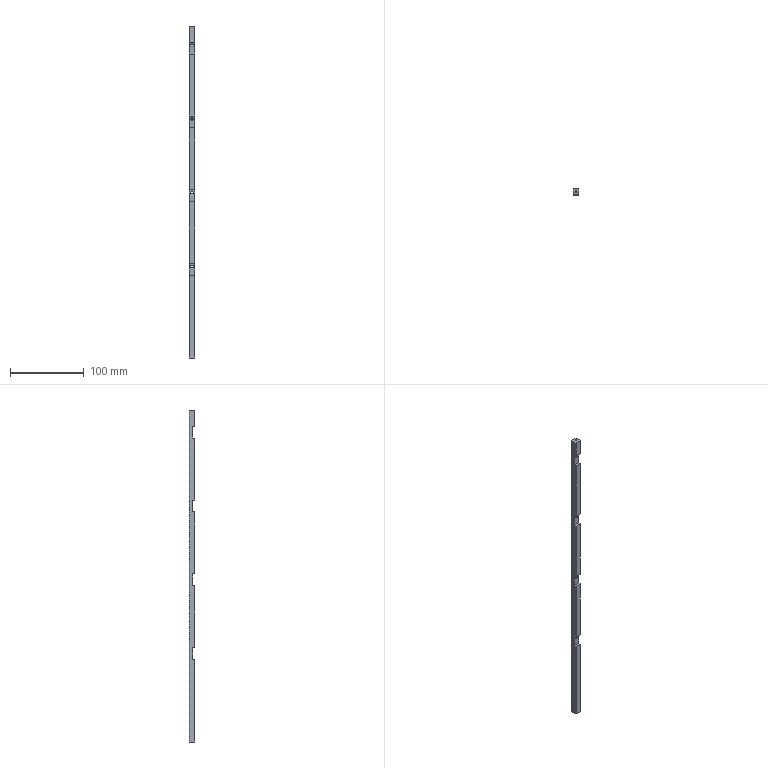Part | SolidWorks | features HoleWzd 3, ICE 2, Extrusion 1 | 1 solid | 50 faces | box 8 x 8 x 450 mm | volume 26809 mm3 | plane 26 | cylinder 20 | cone 4 | commonest cylinder face diameters 3.4 x8 6 x8 2.5 x4
STEP:
#1=CARTESIAN_POINT('',(0.,2.,121.));
#2=VERTEX_POINT('',#1);
#3=CARTESIAN_POINT('',(0.,2.,127.));
#4=VERTEX_POINT('',#3);
#5=CARTESIAN_POINT('',(0.,2.,124.));
#6=DIRECTION('',(0.,1.,0.));
#7=DIRECTION('',(0.,0.,1.));
#8=AXIS2_PLACEMENT_3D('',#5,#6,#7);
#9=CIRCLE('',#8,3.);
#10=EDGE_CURVE('',#2,#4,#9,.T.);
#11=ORIENTED_EDGE('',*,*,#10,.F.);
#12=CARTESIAN_POINT('',(0.,4.,121.));
#13=VERTEX_POINT('',#12);
#14=CARTESIAN_POINT('',(0.,4.,121.));
#15=DIRECTION('',(0.,1.,0.));
#16=VECTOR('',#15,1000.);
#17=LINE('',#14,#16);
#18=EDGE_CURVE('',#2,#13,#17,.T.);
#19=ORIENTED_EDGE('',*,*,#18,.T.);
#20=CARTESIAN_POINT('',(0.,4.,127.));
#21=VERTEX_POINT('',#20);
#22=CARTESIAN_POINT('',(0.,4.,124.));
#23=DIRECTION('',(0.,1.,0.));
#24=DIRECTION('',(0.,0.,1.));
#25=AXIS2_PLACEMENT_3D('',#22,#23,#24);
#26=CIRCLE('',#25,3.);
#27=EDGE_CURVE('',#13,#21,#26,.T.);
#28=ORIENTED_EDGE('',*,*,#27,.T.);
#29=CARTESIAN_POINT('',(0.,4.,127.));
#30=DIRECTION('',(0.,1.,0.));
#31=VECTOR('',#30,1000.);
#32=LINE('',#29,#31);
#33=EDGE_CURVE('',#4,#21,#32,.T.);
#34=ORIENTED_EDGE('',*,*,#33,.F.);
#35=EDGE_LOOP('',(#11,#19,#28,#34));
#36=FACE_OUTER_BOUND('',#35,.T.);
#37=CARTESIAN_POINT('',(0.,4.,124.));
#38=DIRECTION('',(0.,1.,0.));
#39=DIRECTION('',(0.,0.,1.));
#40=AXIS2_PLACEMENT_3D('',#37,#38,#39);
#41=CYLINDRICAL_SURFACE('',#40,3.);
#42=ADVANCED_FACE('',(#36),#41,.F.);
#43=CARTESIAN_POINT('',(0.,-1.,122.3));
#44=VERTEX_POINT('',#43);
#45=CARTESIAN_POINT('',(0.,-1.,125.7));
#46=VERTEX_POINT('',#45);
#47=CARTESIAN_POINT('',(0.,-1.,124.));
#48=DIRECTION('',(0.,1.,0.));
#49=DIRECTION('',(-1.,0.,0.));
#50=AXIS2_PLACEMENT_3D('',#47,#48,#49);
#51=CIRCLE('',#50,1.7);
#52=EDGE_CURVE('',#44,#46,#51,.T.);
#53=ORIENTED_EDGE('',*,*,#52,.F.);
#54=CARTESIAN_POINT('',(0.,2.,122.3));
#55=VERTEX_POINT('',#54);
#56=CARTESIAN_POINT('',(0.,4.,122.3));
#57=DIRECTION('',(0.,1.,0.));
#58=VECTOR('',#57,1000.);
#59=LINE('',#56,#58);
#60=EDGE_CURVE('',#44,#55,#59,.T.);
#61=ORIENTED_EDGE('',*,*,#60,.T.);
#62=CARTESIAN_POINT('',(0.,2.,125.7));
#63=VERTEX_POINT('',#62);
#64=CARTESIAN_POINT('',(0.,2.,124.));
#65=DIRECTION('',(0.,1.,0.));
#66=DIRECTION('',(0.,0.,1.));
#67=AXIS2_PLACEMENT_3D('',#64,#65,#66);
#68=CIRCLE('',#67,1.7);
#69=EDGE_CURVE('',#55,#63,#68,.T.);
#70=ORIENTED_EDGE('',*,*,#69,.T.);
#71=CARTESIAN_POINT('',(0.,4.,125.7));
#72=DIRECTION('',(0.,1.,0.));
#73=VECTOR('',#72,1000.);
#74=LINE('',#71,#73);
#75=EDGE_CURVE('',#46,#63,#74,.T.);
#76=ORIENTED_EDGE('',*,*,#75,.F.);
#77=EDGE_LOOP('',(#53,#61,#70,#76));
#78=FACE_OUTER_BOUND('',#77,.T.);
#79=CARTESIAN_POINT('',(0.,4.,124.));
#80=DIRECTION('',(0.,1.,0.));
#81=DIRECTION('',(0.,0.,1.));
#82=AXIS2_PLACEMENT_3D('',#79,#80,#81);
#83=CYLINDRICAL_SURFACE('',#82,1.7);
#84=ADVANCED_FACE('',(#78),#83,.F.);
#85=CARTESIAN_POINT('',(0.,2.,221.));
#86=VERTEX_POINT('',#85);
#87=CARTESIAN_POINT('',(0.,2.,227.));
#88=VERTEX_POINT('',#87);
#89=CARTESIAN_POINT('',(0.,2.,224.));
#90=DIRECTION('',(0.,1.,0.));
#91=DIRECTION('',(0.,0.,1.));
#92=AXIS2_PLACEMENT_3D('',#89,#90,#91);
#93=CIRCLE('',#92,3.);
#94=EDGE_CURVE('',#86,#88,#93,.T.);
#95=ORIENTED_EDGE('',*,*,#94,.F.);
#96=CARTESIAN_POINT('',(0.,4.,221.));
#97=VERTEX_POINT('',#96);
#98=CARTESIAN_POINT('',(0.,4.,221.));
#99=DIRECTION('',(0.,1.,0.));
#100=VECTOR('',#99,1000.);
#101=LINE('',#98,#100);
#102=EDGE_CURVE('',#86,#97,#101,.T.);
#103=ORIENTED_EDGE('',*,*,#102,.T.);
#104=CARTESIAN_POINT('',(0.,4.,227.));
#105=VERTEX_POINT('',#104);
#106=CARTESIAN_POINT('',(0.,4.,224.));
#107=DIRECTION('',(0.,1.,0.));
#108=DIRECTION('',(0.,0.,1.));
#109=AXIS2_PLACEMENT_3D('',#106,#107,#108);
#110=CIRCLE('',#109,3.);
#111=EDGE_CURVE('',#97,#105,#110,.T.);
#112=ORIENTED_EDGE('',*,*,#111,.T.);
#113=CARTESIAN_POINT('',(0.,4.,227.));
#114=DIRECTION('',(0.,1.,0.));
#115=VECTOR('',#114,1000.);
#116=LINE('',#113,#115);
#117=EDGE_CURVE('',#88,#105,#116,.T.);
#118=ORIENTED_EDGE('',*,*,#117,.F.);
#119=EDGE_LOOP('',(#95,#103,#112,#118));
#120=FACE_OUTER_BOUND('',#119,.T.);
#121=CARTESIAN_POINT('',(0.,4.,224.));
#122=DIRECTION('',(0.,1.,0.));
#123=DIRECTION('',(0.,0.,1.));
#124=AXIS2_PLACEMENT_3D('',#121,#122,#123);
#125=CYLINDRICAL_SURFACE('',#124,3.);
#126=ADVANCED_FACE('',(#120),#125,.F.);
#127=CARTESIAN_POINT('',(0.,-1.,222.3));
#128=VERTEX_POINT('',#127);
#129=CARTESIAN_POINT('',(0.,-1.,225.7));
#130=VERTEX_POINT('',#129);
#131=CARTESIAN_POINT('',(0.,-1.,224.));
#132=DIRECTION('',(0.,1.,0.));
#133=DIRECTION('',(-1.,0.,0.));
#134=AXIS2_PLACEMENT_3D('',#131,#132,#133);
#135=CIRCLE('',#134,1.7);
#136=EDGE_CURVE('',#128,#130,#135,.T.);
#137=ORIENTED_EDGE('',*,*,#136,.F.);
#138=CARTESIAN_POINT('',(0.,2.,222.3));
#139=VERTEX_POINT('',#138);
#140=CARTESIAN_POINT('',(0.,4.,222.3));
#141=DIRECTION('',(0.,1.,0.));
#142=VECTOR('',#141,1000.);
#143=LINE('',#140,#142);
#144=EDGE_CURVE('',#128,#139,#143,.T.);
#145=ORIENTED_EDGE('',*,*,#144,.T.);
#146=CARTESIAN_POINT('',(0.,2.,225.7));
#147=VERTEX_POINT('',#146);
#148=CARTESIAN_POINT('',(0.,2.,224.));
#149=DIRECTION('',(0.,1.,0.));
#150=DIRECTION('',(0.,0.,1.));
#151=AXIS2_PLACEMENT_3D('',#148,#149,#150);
#152=CIRCLE('',#151,1.7);
#153=EDGE_CURVE('',#139,#147,#152,.T.);
#154=ORIENTED_EDGE('',*,*,#153,.T.);
#155=CARTESIAN_POINT('',(0.,4.,225.7));
#156=DIRECTION('',(0.,1.,0.));
#157=VECTOR('',#156,1000.);
#158=LINE('',#155,#157);
#159=EDGE_CURVE('',#130,#147,#158,.T.);
#160=ORIENTED_EDGE('',*,*,#159,.F.);
#161=EDGE_LOOP('',(#137,#145,#154,#160));
#162=FACE_OUTER_BOUND('',#161,.T.);
#163=CARTESIAN_POINT('',(0.,4.,224.));
#164=DIRECTION('',(0.,1.,0.));
#165=DIRECTION('',(0.,0.,1.));
#166=AXIS2_PLACEMENT_3D('',#163,#164,#165);
#167=CYLINDRICAL_SURFACE('',#166,1.7);
#168=ADVANCED_FACE('',(#162),#167,.F.);
#169=CARTESIAN_POINT('',(0.,2.,321.));
#170=VERTEX_POINT('',#169);
#171=CARTESIAN_POINT('',(0.,2.,327.));
#172=VERTEX_POINT('',#171);
#173=CARTESIAN_POINT('',(0.,2.,324.));
#174=DIRECTION('',(0.,1.,0.));
#175=DIRECTION('',(0.,0.,1.));
#176=AXIS2_PLACEMENT_3D('',#173,#174,#175);
#177=CIRCLE('',#176,3.);
#178=EDGE_CURVE('',#170,#172,#177,.T.);
#179=ORIENTED_EDGE('',*,*,#178,.F.);
#180=CARTESIAN_POINT('',(0.,4.,321.));
#181=VERTEX_POINT('',#180);
#182=CARTESIAN_POINT('',(0.,4.,321.));
#183=DIRECTION('',(0.,1.,0.));
#184=VECTOR('',#183,1000.);
#185=LINE('',#182,#184);
#186=EDGE_CURVE('',#170,#181,#185,.T.);
#187=ORIENTED_EDGE('',*,*,#186,.T.);
#188=CARTESIAN_POINT('',(0.,4.,327.));
#189=VERTEX_POINT('',#188);
#190=CARTESIAN_POINT('',(0.,4.,324.));
#191=DIRECTION('',(0.,1.,0.));
#192=DIRECTION('',(0.,0.,1.));
#193=AXIS2_PLACEMENT_3D('',#190,#191,#192);
#194=CIRCLE('',#193,3.);
#195=EDGE_CURVE('',#181,#189,#194,.T.);
#196=ORIENTED_EDGE('',*,*,#195,.T.);
#197=CARTESIAN_POINT('',(0.,4.,327.));
#198=DIRECTION('',(0.,1.,0.));
#199=VECTOR('',#198,1000.);
#200=LINE('',#197,#199);
#201=EDGE_CURVE('',#172,#189,#200,.T.);
#202=ORIENTED_EDGE('',*,*,#201,.F.);
#203=EDGE_LOOP('',(#179,#187,#196,#202));
#204=FACE_OUTER_BOUND('',#203,.T.);
#205=CARTESIAN_POINT('',(0.,4.,324.));
#206=DIRECTION('',(0.,1.,0.));
#207=DIRECTION('',(0.,0.,1.));
#208=AXIS2_PLACEMENT_3D('',#205,#206,#207);
#209=CYLINDRICAL_SURFACE('',#208,3.);
#210=ADVANCED_FACE('',(#204),#209,.F.);
#211=CARTESIAN_POINT('',(0.,-1.,322.3));
#212=VERTEX_POINT('',#211);
#213=CARTESIAN_POINT('',(0.,-1.,325.7));
#214=VERTEX_POINT('',#213);
#215=CARTESIAN_POINT('',(0.,-1.,324.));
#216=DIRECTION('',(0.,1.,0.));
#217=DIRECTION('',(0.,0.,1.));
#218=AXIS2_PLACEMENT_3D('',#215,#216,#217);
#219=CIRCLE('',#218,1.7);
#220=EDGE_CURVE('',#212,#214,#219,.T.);
#221=ORIENTED_EDGE('',*,*,#220,.F.);
#222=CARTESIAN_POINT('',(0.,2.,322.3));
#223=VERTEX_POINT('',#222);
#224=CARTESIAN_POINT('',(0.,4.,322.3));
#225=DIRECTION('',(0.,1.,0.));
#226=VECTOR('',#225,1000.);
#227=LINE('',#224,#226);
#228=EDGE_CURVE('',#212,#223,#227,.T.);
#229=ORIENTED_EDGE('',*,*,#228,.T.);
#230=CARTESIAN_POINT('',(0.,2.,325.7));
#231=VERTEX_POINT('',#230);
#232=CARTESIAN_POINT('',(0.,2.,324.));
#233=DIRECTION('',(0.,1.,0.));
#234=DIRECTION('',(0.,0.,1.));
#235=AXIS2_PLACEMENT_3D('',#232,#233,#234);
#236=CIRCLE('',#235,1.7);
#237=EDGE_CURVE('',#223,#231,#236,.T.);
#238=ORIENTED_EDGE('',*,*,#237,.T.);
#239=CARTESIAN_POINT('',(0.,4.,325.7));
#240=DIRECTION('',(0.,1.,0.));
#241=VECTOR('',#240,1000.);
#242=LINE('',#239,#241);
#243=EDGE_CURVE('',#214,#231,#242,.T.);
#244=ORIENTED_EDGE('',*,*,#243,.F.);
#245=EDGE_LOOP('',(#221,#229,#238,#244));
#246=FACE_OUTER_BOUND('',#245,.T.);
#247=CARTESIAN_POINT('',(0.,4.,324.));
#248=DIRECTION('',(0.,1.,0.));
#249=DIRECTION('',(0.,0.,1.));
#250=AXIS2_PLACEMENT_3D('',#247,#248,#249);
#251=CYLINDRICAL_SURFACE('',#250,1.7);
#252=ADVANCED_FACE('',(#246),#251,.F.);
#253=CARTESIAN_POINT('',(0.,2.,421.));
#254=VERTEX_POINT('',#253);
#255=CARTESIAN_POINT('',(0.,2.,427.));
#256=VERTEX_POINT('',#255);
#257=CARTESIAN_POINT('',(0.,2.,424.));
#258=DIRECTION('',(0.,1.,0.));
#259=DIRECTION('',(0.,0.,1.));
#260=AXIS2_PLACEMENT_3D('',#257,#258,#259);
#261=CIRCLE('',#260,3.);
#262=EDGE_CURVE('',#254,#256,#261,.T.);
#263=ORIENTED_EDGE('',*,*,#262,.F.);
#264=CARTESIAN_POINT('',(0.,4.,421.));
#265=VERTEX_POINT('',#264);
#266=CARTESIAN_POINT('',(0.,4.,421.));
#267=DIRECTION('',(0.,1.,0.));
#268=VECTOR('',#267,1000.);
#269=LINE('',#266,#268);
#270=EDGE_CURVE('',#254,#265,#269,.T.);
#271=ORIENTED_EDGE('',*,*,#270,.T.);
#272=CARTESIAN_POINT('',(0.,4.,427.));
#273=VERTEX_POINT('',#272);
#274=CARTESIAN_POINT('',(0.,4.,424.));
#275=DIRECTION('',(0.,1.,0.));
#276=DIRECTION('',(0.,0.,1.));
#277=AXIS2_PLACEMENT_3D('',#274,#275,#276);
#278=CIRCLE('',#277,3.);
#279=EDGE_CURVE('',#265,#273,#278,.T.);
#280=ORIENTED_EDGE('',*,*,#279,.T.);
#281=CARTESIAN_POINT('',(0.,4.,427.));
#282=DIRECTION('',(0.,1.,0.));
#283=VECTOR('',#282,1000.);
#284=LINE('',#281,#283);
#285=EDGE_CURVE('',#256,#273,#284,.T.);
#286=ORIENTED_EDGE('',*,*,#285,.F.);
#287=EDGE_LOOP('',(#263,#271,#280,#286));
#288=FACE_OUTER_BOUND('',#287,.T.);
#289=CARTESIAN_POINT('',(0.,4.,424.));
#290=DIRECTION('',(0.,1.,0.));
#291=DIRECTION('',(0.,0.,1.));
#292=AXIS2_PLACEMENT_3D('',#289,#290,#291);
#293=CYLINDRICAL_SURFACE('',#292,3.);
#294=ADVANCED_FACE('',(#288),#293,.F.);
#295=CARTESIAN_POINT('',(0.,-1.,425.7));
#296=VERTEX_POINT('',#295);
#297=CARTESIAN_POINT('',(0.,-1.,422.3));
#298=VERTEX_POINT('',#297);
#299=CARTESIAN_POINT('',(0.,-1.,424.));
#300=DIRECTION('',(0.,-1.,0.));
#301=DIRECTION('',(0.,0.,-1.));
#302=AXIS2_PLACEMENT_3D('',#299,#300,#301);
#303=CIRCLE('',#302,1.7);
#304=EDGE_CURVE('',#296,#298,#303,.T.);
#305=ORIENTED_EDGE('',*,*,#304,.T.);
#306=CARTESIAN_POINT('',(0.,2.,422.3));
#307=VERTEX_POINT('',#306);
#308=CARTESIAN_POINT('',(0.,4.,422.3));
#309=DIRECTION('',(0.,1.,0.));
#310=VECTOR('',#309,1000.);
#311=LINE('',#308,#310);
#312=EDGE_CURVE('',#298,#307,#311,.T.);
#313=ORIENTED_EDGE('',*,*,#312,.T.);
#314=CARTESIAN_POINT('',(0.,2.,425.7));
#315=VERTEX_POINT('',#314);
#316=CARTESIAN_POINT('',(0.,2.,424.));
#317=DIRECTION('',(0.,1.,0.));
#318=DIRECTION('',(0.,0.,1.));
#319=AXIS2_PLACEMENT_3D('',#316,#317,#318);
#320=CIRCLE('',#319,1.7);
#321=EDGE_CURVE('',#307,#315,#320,.T.);
#322=ORIENTED_EDGE('',*,*,#321,.T.);
#323=CARTESIAN_POINT('',(0.,4.,425.7));
#324=DIRECTION('',(0.,1.,0.));
#325=VECTOR('',#324,1000.);
#326=LINE('',#323,#325);
#327=EDGE_CURVE('',#296,#315,#326,.T.);
#328=ORIENTED_EDGE('',*,*,#327,.F.);
#329=EDGE_LOOP('',(#305,#313,#322,#328));
#330=FACE_OUTER_BOUND('',#329,.T.);
#331=CARTESIAN_POINT('',(0.,4.,424.));
#332=DIRECTION('',(0.,1.,0.));
#333=DIRECTION('',(0.,0.,1.));
#334=AXIS2_PLACEMENT_3D('',#331,#332,#333);
#335=CYLINDRICAL_SURFACE('',#334,1.7);
#336=ADVANCED_FACE('',(#330),#335,.F.);
#337=CARTESIAN_POINT('',(-1.25,0.,438.));
#338=VERTEX_POINT('',#337);
#339=CARTESIAN_POINT('',(1.25,0.,438.));
#340=VERTEX_POINT('',#339);
#341=CARTESIAN_POINT('',(0.,0.,438.));
#342=DIRECTION('',(0.,0.,1.));
#343=DIRECTION('',(1.,0.,0.));
#344=AXIS2_PLACEMENT_3D('',#341,#342,#343);
#345=CIRCLE('',#344,1.25);
#346=EDGE_CURVE('',#338,#340,#345,.T.);
#347=ORIENTED_EDGE('',*,*,#346,.F.);
#348=CARTESIAN_POINT('',(-1.25,0.,450.));
#349=VERTEX_POINT('',#348);
#350=CARTESIAN_POINT('',(-1.25,0.,450.));
#351=DIRECTION('',(0.,0.,1.));
#352=VECTOR('',#351,1000.);
#353=LINE('',#350,#352);
#354=EDGE_CURVE('',#338,#349,#353,.T.);
#355=ORIENTED_EDGE('',*,*,#354,.T.);
#356=CARTESIAN_POINT('',(1.25,0.,450.));
#357=VERTEX_POINT('',#356);
#358=CARTESIAN_POINT('',(0.,0.,450.));
#359=DIRECTION('',(0.,0.,1.));
#360=DIRECTION('',(1.,0.,0.));
#361=AXIS2_PLACEMENT_3D('',#358,#359,#360);
#362=CIRCLE('',#361,1.25);
#363=EDGE_CURVE('',#349,#357,#362,.T.);
#364=ORIENTED_EDGE('',*,*,#363,.T.);
#365=CARTESIAN_POINT('',(1.25,0.,450.));
#366=DIRECTION('',(0.,0.,1.));
#367=VECTOR('',#366,1000.);
#368=LINE('',#365,#367);
#369=EDGE_CURVE('',#340,#357,#368,.T.);
#370=ORIENTED_EDGE('',*,*,#369,.F.);
#371=EDGE_LOOP('',(#347,#355,#364,#370));
#372=FACE_OUTER_BOUND('',#371,.T.);
#373=CARTESIAN_POINT('',(0.,0.,450.));
#374=DIRECTION('',(0.,0.,1.));
#375=DIRECTION('',(1.,0.,0.));
#376=AXIS2_PLACEMENT_3D('',#373,#374,#375);
#377=CYLINDRICAL_SURFACE('',#376,1.25);
#378=ADVANCED_FACE('',(#372),#377,.F.);
#379=CARTESIAN_POINT('',(0.,0.,437.249));
#380=VERTEX_POINT('',#379);
#381=CARTESIAN_POINT('',(1.25,0.,438.));
#382=DIRECTION('',(0.8572,0.,0.515));
#383=VECTOR('',#382,1000.);
#384=LINE('',#381,#383);
#385=EDGE_CURVE('',#380,#340,#384,.T.);
#386=ORIENTED_EDGE('',*,*,#385,.F.);
#387=CARTESIAN_POINT('',(-1.25,0.,438.));
#388=DIRECTION('',(-0.8572,0.,0.515));
#389=VECTOR('',#388,1000.);
#390=LINE('',#387,#389);
#391=EDGE_CURVE('',#380,#338,#390,.T.);
#392=ORIENTED_EDGE('',*,*,#391,.T.);
#393=ORIENTED_EDGE('',*,*,#346,.T.);
#394=EDGE_LOOP('',(#386,#392,#393));
#395=FACE_OUTER_BOUND('',#394,.T.);
#396=CARTESIAN_POINT('',(0.,0.,438.));
#397=DIRECTION('',(0.,0.,1.));
#398=DIRECTION('',(1.,0.,0.));
#399=AXIS2_PLACEMENT_3D('',#396,#397,#398);
#400=CONICAL_SURFACE('',#399,1.25,1.03);
#401=ADVANCED_FACE('',(#395),#400,.F.);
#402=CARTESIAN_POINT('',(1.25,0.,12.));
#403=VERTEX_POINT('',#402);
#404=CARTESIAN_POINT('',(-1.25,0.,12.));
#405=VERTEX_POINT('',#404);
#406=CARTESIAN_POINT('',(0.,0.,12.));
#407=DIRECTION('',(0.,0.,-1.));
#408=DIRECTION('',(-1.,0.,0.));
#409=AXIS2_PLACEMENT_3D('',#406,#407,#408);
#410=CIRCLE('',#409,1.25);
#411=EDGE_CURVE('',#403,#405,#410,.T.);
#412=ORIENTED_EDGE('',*,*,#411,.F.);
#413=CARTESIAN_POINT('',(1.25,0.,0.));
#414=VERTEX_POINT('',#413);
#415=CARTESIAN_POINT('',(1.25,0.,0.));
#416=DIRECTION('',(0.,0.,-1.));
#417=VECTOR('',#416,1000.);
#418=LINE('',#415,#417);
#419=EDGE_CURVE('',#403,#414,#418,.T.);
#420=ORIENTED_EDGE('',*,*,#419,.T.);
#421=CARTESIAN_POINT('',(-1.25,0.,0.));
#422=VERTEX_POINT('',#421);
#423=CARTESIAN_POINT('',(0.,0.,0.));
#424=DIRECTION('',(0.,0.,-1.));
#425=DIRECTION('',(-1.,0.,0.));
#426=AXIS2_PLACEMENT_3D('',#423,#424,#425);
#427=CIRCLE('',#426,1.25);
#428=EDGE_CURVE('',#414,#422,#427,.T.);
#429=ORIENTED_EDGE('',*,*,#428,.T.);
#430=CARTESIAN_POINT('',(-1.25,0.,0.));
#431=DIRECTION('',(0.,0.,-1.));
#432=VECTOR('',#431,1000.);
#433=LINE('',#430,#432);
#434=EDGE_CURVE('',#405,#422,#433,.T.);
#435=ORIENTED_EDGE('',*,*,#434,.F.);
#436=EDGE_LOOP('',(#412,#420,#429,#435));
#437=FACE_OUTER_BOUND('',#436,.T.);
#438=CARTESIAN_POINT('',(0.,0.,0.));
#439=DIRECTION('',(0.,0.,-1.));
#440=DIRECTION('',(-1.,0.,0.));
#441=AXIS2_PLACEMENT_3D('',#438,#439,#440);
#442=CYLINDRICAL_SURFACE('',#441,1.25);
#443=ADVANCED_FACE('',(#437),#442,.F.);
#444=CARTESIAN_POINT('',(0.,0.,12.751));
#445=VERTEX_POINT('',#444);
#446=CARTESIAN_POINT('',(-1.25,0.,12.));
#447=DIRECTION('',(-0.8572,0.,-0.515));
#448=VECTOR('',#447,1000.);
#449=LINE('',#446,#448);
#450=EDGE_CURVE('',#445,#405,#449,.T.);
#451=ORIENTED_EDGE('',*,*,#450,.F.);
#452=CARTESIAN_POINT('',(1.25,0.,12.));
#453=DIRECTION('',(0.8572,0.,-0.515));
#454=VECTOR('',#453,1000.);
#455=LINE('',#452,#454);
#456=EDGE_CURVE('',#445,#403,#455,.T.);
#457=ORIENTED_EDGE('',*,*,#456,.T.);
#458=ORIENTED_EDGE('',*,*,#411,.T.);
#459=EDGE_LOOP('',(#451,#457,#458));
#460=FACE_OUTER_BOUND('',#459,.T.);
#461=CARTESIAN_POINT('',(0.,0.,12.));
#462=DIRECTION('',(0.,0.,-1.));
#463=DIRECTION('',(-1.,0.,0.));
#464=AXIS2_PLACEMENT_3D('',#461,#462,#463);
#465=CONICAL_SURFACE('',#464,1.25,1.03);
#466=ADVANCED_FACE('',(#460),#465,.F.);
#467=CARTESIAN_POINT('',(-4.,-4.,212.));
#468=VERTEX_POINT('',#467);
#469=CARTESIAN_POINT('',(-4.,-4.,128.));
#470=VERTEX_POINT('',#469);
#471=CARTESIAN_POINT('',(-4.,-4.,450.));
#472=DIRECTION('',(0.,0.,-1.));
#473=VECTOR('',#472,1000.);
#474=LINE('',#471,#473);
#475=EDGE_CURVE('',#468,#470,#474,.T.);
#476=ORIENTED_EDGE('',*,*,#475,.T.);
#477=CARTESIAN_POINT('',(4.,-4.,128.));
#478=VERTEX_POINT('',#477);
#479=CARTESIAN_POINT('',(-4.,-4.,128.));
#480=DIRECTION('',(1.,0.,0.));
#481=VECTOR('',#480,1000.);
#482=LINE('',#479,#481);
#483=EDGE_CURVE('',#470,#478,#482,.T.);
#484=ORIENTED_EDGE('',*,*,#483,.T.);
#485=CARTESIAN_POINT('',(4.,-4.,212.));
#486=VERTEX_POINT('',#485);
#487=CARTESIAN_POINT('',(4.,-4.,450.));
#488=DIRECTION('',(0.,0.,-1.));
#489=VECTOR('',#488,1000.);
#490=LINE('',#487,#489);
#491=EDGE_CURVE('',#486,#478,#490,.T.);
#492=ORIENTED_EDGE('',*,*,#491,.F.);
#493=CARTESIAN_POINT('',(-4.,-4.,212.));
#494=DIRECTION('',(1.,0.,0.));
#495=VECTOR('',#494,1000.);
#496=LINE('',#493,#495);
#497=EDGE_CURVE('',#468,#486,#496,.T.);
#498=ORIENTED_EDGE('',*,*,#497,.F.);
#499=EDGE_LOOP('',(#476,#484,#492,#498));
#500=FACE_OUTER_BOUND('',#499,.T.);
#501=CARTESIAN_POINT('',(-4.,-4.,450.));
#502=DIRECTION('',(0.,1.,0.));
#503=DIRECTION('',(0.,0.,1.));
#504=AXIS2_PLACEMENT_3D('',#501,#502,#503);
#505=PLANE('',#504);
#506=ADVANCED_FACE('',(#500),#505,.F.);
#507=CARTESIAN_POINT('',(-4.,-4.,312.));
#508=VERTEX_POINT('',#507);
#509=CARTESIAN_POINT('',(-4.,-4.,228.));
#510=VERTEX_POINT('',#509);
#511=CARTESIAN_POINT('',(-4.,-4.,450.));
#512=DIRECTION('',(0.,0.,-1.));
#513=VECTOR('',#512,1000.);
#514=LINE('',#511,#513);
#515=EDGE_CURVE('',#508,#510,#514,.T.);
#516=ORIENTED_EDGE('',*,*,#515,.T.);
#517=CARTESIAN_POINT('',(4.,-4.,228.));
#518=VERTEX_POINT('',#517);
#519=CARTESIAN_POINT('',(-4.,-4.,228.));
#520=DIRECTION('',(1.,0.,0.));
#521=VECTOR('',#520,1000.);
#522=LINE('',#519,#521);
#523=EDGE_CURVE('',#510,#518,#522,.T.);
#524=ORIENTED_EDGE('',*,*,#523,.T.);
#525=CARTESIAN_POINT('',(4.,-4.,312.));
#526=VERTEX_POINT('',#525);
#527=CARTESIAN_POINT('',(4.,-4.,450.));
#528=DIRECTION('',(0.,0.,-1.));
#529=VECTOR('',#528,1000.);
#530=LINE('',#527,#529);
#531=EDGE_CURVE('',#526,#518,#530,.T.);
#532=ORIENTED_EDGE('',*,*,#531,.F.);
#533=CARTESIAN_POINT('',(-4.,-4.,312.));
#534=DIRECTION('',(1.,0.,0.));
#535=VECTOR('',#534,1000.);
#536=LINE('',#533,#535);
#537=EDGE_CURVE('',#508,#526,#536,.T.);
#538=ORIENTED_EDGE('',*,*,#537,.F.);
#539=EDGE_LOOP('',(#516,#524,#532,#538));
#540=FACE_OUTER_BOUND('',#539,.T.);
#541=CARTESIAN_POINT('',(-4.,-4.,450.));
#542=DIRECTION('',(0.,1.,0.));
#543=DIRECTION('',(0.,0.,1.));
#544=AXIS2_PLACEMENT_3D('',#541,#542,#543);
#545=PLANE('',#544);
#546=ADVANCED_FACE('',(#540),#545,.F.);
#547=CARTESIAN_POINT('',(4.,-4.,112.));
#548=VERTEX_POINT('',#547);
#549=CARTESIAN_POINT('',(4.,-4.,0.));
#550=VERTEX_POINT('',#549);
#551=CARTESIAN_POINT('',(4.,-4.,450.));
#552=DIRECTION('',(0.,0.,-1.));
#553=VECTOR('',#552,1000.);
#554=LINE('',#551,#553);
#555=EDGE_CURVE('',#548,#550,#554,.T.);
#556=ORIENTED_EDGE('',*,*,#555,.F.);
#557=CARTESIAN_POINT('',(-4.,-4.,112.));
#558=VERTEX_POINT('',#557);
#559=CARTESIAN_POINT('',(-4.,-4.,112.));
#560=DIRECTION('',(1.,0.,0.));
#561=VECTOR('',#560,1000.);
#562=LINE('',#559,#561);
#563=EDGE_CURVE('',#558,#548,#562,.T.);
#564=ORIENTED_EDGE('',*,*,#563,.F.);
#565=CARTESIAN_POINT('',(-4.,-4.,0.));
#566=VERTEX_POINT('',#565);
#567=CARTESIAN_POINT('',(-4.,-4.,450.));
#568=DIRECTION('',(0.,0.,-1.));
#569=VECTOR('',#568,1000.);
#570=LINE('',#567,#569);
#571=EDGE_CURVE('',#558,#566,#570,.T.);
#572=ORIENTED_EDGE('',*,*,#571,.T.);
#573=CARTESIAN_POINT('',(-4.,-4.,0.));
#574=DIRECTION('',(1.,0.,0.));
#575=VECTOR('',#574,1000.);
#576=LINE('',#573,#575);
#577=EDGE_CURVE('',#566,#550,#576,.T.);
#578=ORIENTED_EDGE('',*,*,#577,.T.);
#579=EDGE_LOOP('',(#556,#564,#572,#578));
#580=FACE_OUTER_BOUND('',#579,.T.);
#581=CARTESIAN_POINT('',(-4.,-4.,450.));
#582=DIRECTION('',(0.,1.,0.));
#583=DIRECTION('',(0.,0.,1.));
#584=AXIS2_PLACEMENT_3D('',#581,#582,#583);
#585=PLANE('',#584);
#586=ADVANCED_FACE('',(#580),#585,.F.);
#587=CARTESIAN_POINT('',(-4.,-4.,450.));
#588=VERTEX_POINT('',#587);
#589=CARTESIAN_POINT('',(-4.,-4.,428.));
#590=VERTEX_POINT('',#589);
#591=CARTESIAN_POINT('',(-4.,-4.,450.));
#592=DIRECTION('',(0.,0.,-1.));
#593=VECTOR('',#592,1000.);
#594=LINE('',#591,#593);
#595=EDGE_CURVE('',#588,#590,#594,.T.);
#596=ORIENTED_EDGE('',*,*,#595,.T.);
#597=CARTESIAN_POINT('',(4.,-4.,428.));
#598=VERTEX_POINT('',#597);
#599=CARTESIAN_POINT('',(-4.,-4.,428.));
#600=DIRECTION('',(-1.,0.,0.));
#601=VECTOR('',#600,1000.);
#602=LINE('',#599,#601);
#603=EDGE_CURVE('',#598,#590,#602,.T.);
#604=ORIENTED_EDGE('',*,*,#603,.F.);
#605=CARTESIAN_POINT('',(4.,-4.,450.));
#606=VERTEX_POINT('',#605);
#607=CARTESIAN_POINT('',(4.,-4.,450.));
#608=DIRECTION('',(0.,0.,-1.));
#609=VECTOR('',#608,1000.);
#610=LINE('',#607,#609);
#611=EDGE_CURVE('',#606,#598,#610,.T.);
#612=ORIENTED_EDGE('',*,*,#611,.F.);
#613=CARTESIAN_POINT('',(-4.,-4.,450.));
#614=DIRECTION('',(1.,0.,0.));
#615=VECTOR('',#614,1000.);
#616=LINE('',#613,#615);
#617=EDGE_CURVE('',#588,#606,#616,.T.);
#618=ORIENTED_EDGE('',*,*,#617,.F.);
#619=EDGE_LOOP('',(#596,#604,#612,#618));
#620=FACE_OUTER_BOUND('',#619,.T.);
#621=CARTESIAN_POINT('',(-4.,-4.,450.));
#622=DIRECTION('',(0.,1.,0.));
#623=DIRECTION('',(0.,0.,1.));
#624=AXIS2_PLACEMENT_3D('',#621,#622,#623);
#625=PLANE('',#624);
#626=ADVANCED_FACE('',(#620),#625,.F.);
#627=ORIENTED_EDGE('',*,*,#491,.T.);
#628=CARTESIAN_POINT('',(4.,-1.,128.));
#629=VERTEX_POINT('',#628);
#630=CARTESIAN_POINT('',(4.,-4.,128.));
#631=DIRECTION('',(0.,-1.,0.));
#632=VECTOR('',#631,1000.);
#633=LINE('',#630,#632);
#634=EDGE_CURVE('',#629,#478,#633,.T.);
#635=ORIENTED_EDGE('',*,*,#634,.F.);
#636=CARTESIAN_POINT('',(4.,-1.,112.));
#637=VERTEX_POINT('',#636);
#638=CARTESIAN_POINT('',(4.,-1.,128.));
#639=DIRECTION('',(0.,0.,1.));
#640=VECTOR('',#639,1000.);
#641=LINE('',#638,#640);
#642=EDGE_CURVE('',#637,#629,#641,.T.);
#643=ORIENTED_EDGE('',*,*,#642,.F.);
#644=CARTESIAN_POINT('',(4.,-4.,112.));
#645=DIRECTION('',(0.,1.,0.));
#646=VECTOR('',#645,1000.);
#647=LINE('',#644,#646);
#648=EDGE_CURVE('',#548,#637,#647,.T.);
#649=ORIENTED_EDGE('',*,*,#648,.F.);
#650=ORIENTED_EDGE('',*,*,#555,.T.);
#651=CARTESIAN_POINT('',(4.,4.,0.));
#652=VERTEX_POINT('',#651);
#653=CARTESIAN_POINT('',(4.,4.,0.));
#654=DIRECTION('',(0.,1.,0.));
#655=VECTOR('',#654,1000.);
#656=LINE('',#653,#655);
#657=EDGE_CURVE('',#550,#652,#656,.T.);
#658=ORIENTED_EDGE('',*,*,#657,.T.);
#659=CARTESIAN_POINT('',(4.,4.,450.));
#660=VERTEX_POINT('',#659);
#661=CARTESIAN_POINT('',(4.,4.,450.));
#662=DIRECTION('',(0.,0.,-1.));
#663=VECTOR('',#662,1000.);
#664=LINE('',#661,#663);
#665=EDGE_CURVE('',#660,#652,#664,.T.);
#666=ORIENTED_EDGE('',*,*,#665,.F.);
#667=CARTESIAN_POINT('',(4.,4.,450.));
#668=DIRECTION('',(0.,1.,0.));
#669=VECTOR('',#668,1000.);
#670=LINE('',#667,#669);
#671=EDGE_CURVE('',#606,#660,#670,.T.);
#672=ORIENTED_EDGE('',*,*,#671,.F.);
#673=ORIENTED_EDGE('',*,*,#611,.T.);
#674=CARTESIAN_POINT('',(4.,-1.,428.));
#675=VERTEX_POINT('',#674);
#676=CARTESIAN_POINT('',(4.,-1.,428.));
#677=DIRECTION('',(0.,-1.,0.));
#678=VECTOR('',#677,1000.);
#679=LINE('',#676,#678);
#680=EDGE_CURVE('',#675,#598,#679,.T.);
#681=ORIENTED_EDGE('',*,*,#680,.F.);
#682=CARTESIAN_POINT('',(4.,-1.,412.));
#683=VERTEX_POINT('',#682);
#684=CARTESIAN_POINT('',(4.,-1.,428.));
#685=DIRECTION('',(0.,0.,1.));
#686=VECTOR('',#685,1000.);
#687=LINE('',#684,#686);
#688=EDGE_CURVE('',#683,#675,#687,.T.);
#689=ORIENTED_EDGE('',*,*,#688,.F.);
#690=CARTESIAN_POINT('',(4.,-4.,412.));
#691=VERTEX_POINT('',#690);
#692=CARTESIAN_POINT('',(4.,-1.,412.));
#693=DIRECTION('',(0.,-1.,0.));
#694=VECTOR('',#693,1000.);
#695=LINE('',#692,#694);
#696=EDGE_CURVE('',#683,#691,#695,.T.);
#697=ORIENTED_EDGE('',*,*,#696,.T.);
#698=CARTESIAN_POINT('',(4.,-4.,328.));
#699=VERTEX_POINT('',#698);
#700=CARTESIAN_POINT('',(4.,-4.,450.));
#701=DIRECTION('',(0.,0.,-1.));
#702=VECTOR('',#701,1000.);
#703=LINE('',#700,#702);
#704=EDGE_CURVE('',#691,#699,#703,.T.);
#705=ORIENTED_EDGE('',*,*,#704,.T.);
#706=CARTESIAN_POINT('',(4.,-1.,328.));
#707=VERTEX_POINT('',#706);
#708=CARTESIAN_POINT('',(4.,-4.,328.));
#709=DIRECTION('',(0.,-1.,0.));
#710=VECTOR('',#709,1000.);
#711=LINE('',#708,#710);
#712=EDGE_CURVE('',#707,#699,#711,.T.);
#713=ORIENTED_EDGE('',*,*,#712,.F.);
#714=CARTESIAN_POINT('',(4.,-1.,312.));
#715=VERTEX_POINT('',#714);
#716=CARTESIAN_POINT('',(4.,-1.,312.));
#717=DIRECTION('',(0.,0.,1.));
#718=VECTOR('',#717,1000.);
#719=LINE('',#716,#718);
#720=EDGE_CURVE('',#715,#707,#719,.T.);
#721=ORIENTED_EDGE('',*,*,#720,.F.);
#722=CARTESIAN_POINT('',(4.,-4.,312.));
#723=DIRECTION('',(0.,1.,0.));
#724=VECTOR('',#723,1000.);
#725=LINE('',#722,#724);
#726=EDGE_CURVE('',#526,#715,#725,.T.);
#727=ORIENTED_EDGE('',*,*,#726,.F.);
#728=ORIENTED_EDGE('',*,*,#531,.T.);
#729=CARTESIAN_POINT('',(4.,-1.,228.));
#730=VERTEX_POINT('',#729);
#731=CARTESIAN_POINT('',(4.,-4.,228.));
#732=DIRECTION('',(0.,-1.,0.));
#733=VECTOR('',#732,1000.);
#734=LINE('',#731,#733);
#735=EDGE_CURVE('',#730,#518,#734,.T.);
#736=ORIENTED_EDGE('',*,*,#735,.F.);
#737=CARTESIAN_POINT('',(4.,-1.,212.));
#738=VERTEX_POINT('',#737);
#739=CARTESIAN_POINT('',(4.,-1.,228.));
#740=DIRECTION('',(0.,0.,1.));
#741=VECTOR('',#740,1000.);
#742=LINE('',#739,#741);
#743=EDGE_CURVE('',#738,#730,#742,.T.);
#744=ORIENTED_EDGE('',*,*,#743,.F.);
#745=CARTESIAN_POINT('',(4.,-4.,212.));
#746=DIRECTION('',(0.,1.,0.));
#747=VECTOR('',#746,1000.);
#748=LINE('',#745,#747);
#749=EDGE_CURVE('',#486,#738,#748,.T.);
#750=ORIENTED_EDGE('',*,*,#749,.F.);
#751=EDGE_LOOP('',(#627,#635,#643,#649,#650,#658,#666,#672,#673,#681,#689,#697,#705,#713,#721,#727,#728,#736,#744,#750));
#752=FACE_OUTER_BOUND('',#751,.T.);
#753=CARTESIAN_POINT('',(4.,4.,450.));
#754=DIRECTION('',(-1.,0.,0.));
#755=DIRECTION('',(0.,-1.,0.));
#756=AXIS2_PLACEMENT_3D('',#753,#754,#755);
#757=PLANE('',#756);
#758=ADVANCED_FACE('',(#752),#757,.F.);
#759=CARTESIAN_POINT('',(0.,4.,124.));
#760=DIRECTION('',(0.,1.,0.));
#761=DIRECTION('',(0.,0.,1.));
#762=AXIS2_PLACEMENT_3D('',#759,#760,#761);
#763=CIRCLE('',#762,3.);
#764=EDGE_CURVE('',#21,#13,#763,.T.);
#765=ORIENTED_EDGE('',*,*,#764,.F.);
#766=ORIENTED_EDGE('',*,*,#27,.F.);
#767=EDGE_LOOP('',(#765,#766));
#768=FACE_BOUND('',#767,.T.);
#769=CARTESIAN_POINT('',(0.,4.,224.));
#770=DIRECTION('',(0.,1.,0.));
#771=DIRECTION('',(0.,0.,1.));
#772=AXIS2_PLACEMENT_3D('',#769,#770,#771);
#773=CIRCLE('',#772,3.);
#774=EDGE_CURVE('',#105,#97,#773,.T.);
#775=ORIENTED_EDGE('',*,*,#774,.F.);
#776=ORIENTED_EDGE('',*,*,#111,.F.);
#777=EDGE_LOOP('',(#775,#776));
#778=FACE_BOUND('',#777,.T.);
#779=CARTESIAN_POINT('',(0.,4.,324.));
#780=DIRECTION('',(0.,1.,0.));
#781=DIRECTION('',(0.,0.,1.));
#782=AXIS2_PLACEMENT_3D('',#779,#780,#781);
#783=CIRCLE('',#782,3.);
#784=EDGE_CURVE('',#189,#181,#783,.T.);
#785=ORIENTED_EDGE('',*,*,#784,.F.);
#786=ORIENTED_EDGE('',*,*,#195,.F.);
#787=EDGE_LOOP('',(#785,#786));
#788=FACE_BOUND('',#787,.T.);
#789=CARTESIAN_POINT('',(0.,4.,424.));
#790=DIRECTION('',(0.,1.,0.));
#791=DIRECTION('',(0.,0.,1.));
#792=AXIS2_PLACEMENT_3D('',#789,#790,#791);
#793=CIRCLE('',#792,3.);
#794=EDGE_CURVE('',#273,#265,#793,.T.);
#795=ORIENTED_EDGE('',*,*,#794,.F.);
#796=ORIENTED_EDGE('',*,*,#279,.F.);
#797=EDGE_LOOP('',(#795,#796));
#798=FACE_BOUND('',#797,.T.);
#799=CARTESIAN_POINT('',(-4.,4.,0.));
#800=VERTEX_POINT('',#799);
#801=CARTESIAN_POINT('',(-4.,4.,0.));
#802=DIRECTION('',(-1.,0.,0.));
#803=VECTOR('',#802,1000.);
#804=LINE('',#801,#803);
#805=EDGE_CURVE('',#652,#800,#804,.T.);
#806=ORIENTED_EDGE('',*,*,#805,.T.);
#807=CARTESIAN_POINT('',(-4.,4.,450.));
#808=VERTEX_POINT('',#807);
#809=CARTESIAN_POINT('',(-4.,4.,450.));
#810=DIRECTION('',(0.,0.,-1.));
#811=VECTOR('',#810,1000.);
#812=LINE('',#809,#811);
#813=EDGE_CURVE('',#808,#800,#812,.T.);
#814=ORIENTED_EDGE('',*,*,#813,.F.);
#815=CARTESIAN_POINT('',(-4.,4.,450.));
#816=DIRECTION('',(-1.,0.,0.));
#817=VECTOR('',#816,1000.);
#818=LINE('',#815,#817);
#819=EDGE_CURVE('',#660,#808,#818,.T.);
#820=ORIENTED_EDGE('',*,*,#819,.F.);
#821=ORIENTED_EDGE('',*,*,#665,.T.);
#822=EDGE_LOOP('',(#806,#814,#820,#821));
#823=FACE_OUTER_BOUND('',#822,.T.);
#824=CARTESIAN_POINT('',(-4.,4.,450.));
#825=DIRECTION('',(0.,-1.,0.));
#826=DIRECTION('',(0.,0.,-1.));
#827=AXIS2_PLACEMENT_3D('',#824,#825,#826);
#828=PLANE('',#827);
#829=ADVANCED_FACE('',(#768,#778,#788,#798,#823),#828,.F.);
#830=CARTESIAN_POINT('',(-4.,-1.,112.));
#831=VERTEX_POINT('',#830);
#832=CARTESIAN_POINT('',(-4.,-1.,128.));
#833=VERTEX_POINT('',#832);
#834=CARTESIAN_POINT('',(-4.,-1.,128.));
#835=DIRECTION('',(0.,0.,1.));
#836=VECTOR('',#835,1000.);
#837=LINE('',#834,#836);
#838=EDGE_CURVE('',#831,#833,#837,.T.);
#839=ORIENTED_EDGE('',*,*,#838,.T.);
#840=CARTESIAN_POINT('',(-4.,-4.,128.));
#841=DIRECTION('',(0.,-1.,0.));
#842=VECTOR('',#841,1000.);
#843=LINE('',#840,#842);
#844=EDGE_CURVE('',#833,#470,#843,.T.);
#845=ORIENTED_EDGE('',*,*,#844,.T.);
#846=ORIENTED_EDGE('',*,*,#475,.F.);
#847=CARTESIAN_POINT('',(-4.,-1.,212.));
#848=VERTEX_POINT('',#847);
#849=CARTESIAN_POINT('',(-4.,-4.,212.));
#850=DIRECTION('',(0.,1.,0.));
#851=VECTOR('',#850,1000.);
#852=LINE('',#849,#851);
#853=EDGE_CURVE('',#468,#848,#852,.T.);
#854=ORIENTED_EDGE('',*,*,#853,.T.);
#855=CARTESIAN_POINT('',(-4.,-1.,228.));
#856=VERTEX_POINT('',#855);
#857=CARTESIAN_POINT('',(-4.,-1.,228.));
#858=DIRECTION('',(0.,0.,1.));
#859=VECTOR('',#858,1000.);
#860=LINE('',#857,#859);
#861=EDGE_CURVE('',#848,#856,#860,.T.);
#862=ORIENTED_EDGE('',*,*,#861,.T.);
#863=CARTESIAN_POINT('',(-4.,-4.,228.));
#864=DIRECTION('',(0.,-1.,0.));
#865=VECTOR('',#864,1000.);
#866=LINE('',#863,#865);
#867=EDGE_CURVE('',#856,#510,#866,.T.);
#868=ORIENTED_EDGE('',*,*,#867,.T.);
#869=ORIENTED_EDGE('',*,*,#515,.F.);
#870=CARTESIAN_POINT('',(-4.,-1.,312.));
#871=VERTEX_POINT('',#870);
#872=CARTESIAN_POINT('',(-4.,-4.,312.));
#873=DIRECTION('',(0.,1.,0.));
#874=VECTOR('',#873,1000.);
#875=LINE('',#872,#874);
#876=EDGE_CURVE('',#508,#871,#875,.T.);
#877=ORIENTED_EDGE('',*,*,#876,.T.);
#878=CARTESIAN_POINT('',(-4.,-1.,328.));
#879=VERTEX_POINT('',#878);
#880=CARTESIAN_POINT('',(-4.,-1.,312.));
#881=DIRECTION('',(0.,0.,1.));
#882=VECTOR('',#881,1000.);
#883=LINE('',#880,#882);
#884=EDGE_CURVE('',#871,#879,#883,.T.);
#885=ORIENTED_EDGE('',*,*,#884,.T.);
#886=CARTESIAN_POINT('',(-4.,-4.,328.));
#887=VERTEX_POINT('',#886);
#888=CARTESIAN_POINT('',(-4.,-4.,328.));
#889=DIRECTION('',(0.,-1.,0.));
#890=VECTOR('',#889,1000.);
#891=LINE('',#888,#890);
#892=EDGE_CURVE('',#879,#887,#891,.T.);
#893=ORIENTED_EDGE('',*,*,#892,.T.);
#894=CARTESIAN_POINT('',(-4.,-4.,412.));
#895=VERTEX_POINT('',#894);
#896=CARTESIAN_POINT('',(-4.,-4.,450.));
#897=DIRECTION('',(0.,0.,-1.));
#898=VECTOR('',#897,1000.);
#899=LINE('',#896,#898);
#900=EDGE_CURVE('',#895,#887,#899,.T.);
#901=ORIENTED_EDGE('',*,*,#900,.F.);
#902=CARTESIAN_POINT('',(-4.,-1.,412.));
#903=VERTEX_POINT('',#902);
#904=CARTESIAN_POINT('',(-4.,-1.,412.));
#905=DIRECTION('',(0.,-1.,0.));
#906=VECTOR('',#905,1000.);
#907=LINE('',#904,#906);
#908=EDGE_CURVE('',#903,#895,#907,.T.);
#909=ORIENTED_EDGE('',*,*,#908,.F.);
#910=CARTESIAN_POINT('',(-4.,-1.,428.));
#911=VERTEX_POINT('',#910);
#912=CARTESIAN_POINT('',(-4.,-1.,428.));
#913=DIRECTION('',(0.,0.,-1.));
#914=VECTOR('',#913,1000.);
#915=LINE('',#912,#914);
#916=EDGE_CURVE('',#911,#903,#915,.T.);
#917=ORIENTED_EDGE('',*,*,#916,.F.);
#918=CARTESIAN_POINT('',(-4.,-1.,428.));
#919=DIRECTION('',(0.,-1.,0.));
#920=VECTOR('',#919,1000.);
#921=LINE('',#918,#920);
#922=EDGE_CURVE('',#911,#590,#921,.T.);
#923=ORIENTED_EDGE('',*,*,#922,.T.);
#924=ORIENTED_EDGE('',*,*,#595,.F.);
#925=CARTESIAN_POINT('',(-4.,4.,450.));
#926=DIRECTION('',(0.,-1.,0.));
#927=VECTOR('',#926,1000.);
#928=LINE('',#925,#927);
#929=EDGE_CURVE('',#808,#588,#928,.T.);
#930=ORIENTED_EDGE('',*,*,#929,.F.);
#931=ORIENTED_EDGE('',*,*,#813,.T.);
#932=CARTESIAN_POINT('',(-4.,4.,0.));
#933=DIRECTION('',(0.,-1.,0.));
#934=VECTOR('',#933,1000.);
#935=LINE('',#932,#934);
#936=EDGE_CURVE('',#800,#566,#935,.T.);
#937=ORIENTED_EDGE('',*,*,#936,.T.);
#938=ORIENTED_EDGE('',*,*,#571,.F.);
#939=CARTESIAN_POINT('',(-4.,-4.,112.));
#940=DIRECTION('',(0.,1.,0.));
#941=VECTOR('',#940,1000.);
#942=LINE('',#939,#941);
#943=EDGE_CURVE('',#558,#831,#942,.T.);
#944=ORIENTED_EDGE('',*,*,#943,.T.);
#945=EDGE_LOOP('',(#839,#845,#846,#854,#862,#868,#869,#877,#885,#893,#901,#909,#917,#923,#924,#930,#931,#937,#938,#944));
#946=FACE_OUTER_BOUND('',#945,.T.);
#947=CARTESIAN_POINT('',(-4.,4.,450.));
#948=DIRECTION('',(1.,0.,0.));
#949=DIRECTION('',(0.,1.,0.));
#950=AXIS2_PLACEMENT_3D('',#947,#948,#949);
#951=PLANE('',#950);
#952=ADVANCED_FACE('',(#946),#951,.F.);
#953=ORIENTED_EDGE('',*,*,#900,.T.);
#954=CARTESIAN_POINT('',(-4.,-4.,328.));
#955=DIRECTION('',(1.,0.,0.));
#956=VECTOR('',#955,1000.);
#957=LINE('',#954,#956);
#958=EDGE_CURVE('',#887,#699,#957,.T.);
#959=ORIENTED_EDGE('',*,*,#958,.T.);
#960=ORIENTED_EDGE('',*,*,#704,.F.);
#961=CARTESIAN_POINT('',(-4.,-4.,412.));
#962=DIRECTION('',(1.,0.,0.));
#963=VECTOR('',#962,1000.);
#964=LINE('',#961,#963);
#965=EDGE_CURVE('',#895,#691,#964,.T.);
#966=ORIENTED_EDGE('',*,*,#965,.F.);
#967=EDGE_LOOP('',(#953,#959,#960,#966));
#968=FACE_OUTER_BOUND('',#967,.T.);
#969=CARTESIAN_POINT('',(-4.,-4.,450.));
#970=DIRECTION('',(0.,1.,0.));
#971=DIRECTION('',(0.,0.,1.));
#972=AXIS2_PLACEMENT_3D('',#969,#970,#971);
#973=PLANE('',#972);
#974=ADVANCED_FACE('',(#968),#973,.F.);
#975=CARTESIAN_POINT('',(0.,0.,450.));
#976=DIRECTION('',(0.,0.,1.));
#977=DIRECTION('',(1.,0.,0.));
#978=AXIS2_PLACEMENT_3D('',#975,#976,#977);
#979=CIRCLE('',#978,1.25);
#980=EDGE_CURVE('',#357,#349,#979,.T.);
#981=ORIENTED_EDGE('',*,*,#980,.F.);
#982=ORIENTED_EDGE('',*,*,#363,.F.);
#983=EDGE_LOOP('',(#981,#982));
#984=FACE_BOUND('',#983,.T.);
#985=ORIENTED_EDGE('',*,*,#671,.T.);
#986=ORIENTED_EDGE('',*,*,#819,.T.);
#987=ORIENTED_EDGE('',*,*,#929,.T.);
#988=ORIENTED_EDGE('',*,*,#617,.T.);
#989=EDGE_LOOP('',(#985,#986,#987,#988));
#990=FACE_OUTER_BOUND('',#989,.T.);
#991=CARTESIAN_POINT('',(0.,0.,450.));
#992=DIRECTION('',(0.,0.,1.));
#993=DIRECTION('',(1.,0.,0.));
#994=AXIS2_PLACEMENT_3D('',#991,#992,#993);
#995=PLANE('',#994);
#996=ADVANCED_FACE('',(#984,#990),#995,.T.);
#997=CARTESIAN_POINT('',(0.,0.,0.));
#998=DIRECTION('',(0.,0.,-1.));
#999=DIRECTION('',(-1.,0.,0.));
#1000=AXIS2_PLACEMENT_3D('',#997,#998,#999);
#1001=CIRCLE('',#1000,1.25);
#1002=EDGE_CURVE('',#422,#414,#1001,.T.);
#1003=ORIENTED_EDGE('',*,*,#1002,.F.);
#1004=ORIENTED_EDGE('',*,*,#428,.F.);
#1005=EDGE_LOOP('',(#1003,#1004));
#1006=FACE_BOUND('',#1005,.T.);
#1007=ORIENTED_EDGE('',*,*,#657,.F.);
#1008=ORIENTED_EDGE('',*,*,#577,.F.);
#1009=ORIENTED_EDGE('',*,*,#936,.F.);
#1010=ORIENTED_EDGE('',*,*,#805,.F.);
#1011=EDGE_LOOP('',(#1007,#1008,#1009,#1010));
#1012=FACE_OUTER_BOUND('',#1011,.T.);
#1013=CARTESIAN_POINT('',(0.,0.,0.));
#1014=DIRECTION('',(0.,0.,1.));
#1015=DIRECTION('',(1.,0.,0.));
#1016=AXIS2_PLACEMENT_3D('',#1013,#1014,#1015);
#1017=PLANE('',#1016);
#1018=ADVANCED_FACE('',(#1006,#1012),#1017,.F.);
#1019=ORIENTED_EDGE('',*,*,#603,.T.);
#1020=ORIENTED_EDGE('',*,*,#922,.F.);
#1021=CARTESIAN_POINT('',(-4.,-1.,428.));
#1022=DIRECTION('',(-1.,0.,0.));
#1023=VECTOR('',#1022,1000.);
#1024=LINE('',#1021,#1023);
#1025=EDGE_CURVE('',#675,#911,#1024,.T.);
#1026=ORIENTED_EDGE('',*,*,#1025,.F.);
#1027=ORIENTED_EDGE('',*,*,#680,.T.);
#1028=EDGE_LOOP('',(#1019,#1020,#1026,#1027));
#1029=FACE_OUTER_BOUND('',#1028,.T.);
#1030=CARTESIAN_POINT('',(-4.,-1.,428.));
#1031=DIRECTION('',(0.,0.,1.));
#1032=DIRECTION('',(1.,0.,0.));
#1033=AXIS2_PLACEMENT_3D('',#1030,#1031,#1032);
#1034=PLANE('',#1033);
#1035=ADVANCED_FACE('',(#1029),#1034,.F.);
#1036=ORIENTED_EDGE('',*,*,#965,.T.);
#1037=ORIENTED_EDGE('',*,*,#696,.F.);
#1038=CARTESIAN_POINT('',(-4.,-1.,412.));
#1039=DIRECTION('',(1.,0.,0.));
#1040=VECTOR('',#1039,1000.);
#1041=LINE('',#1038,#1040);
#1042=EDGE_CURVE('',#903,#683,#1041,.T.);
#1043=ORIENTED_EDGE('',*,*,#1042,.F.);
#1044=ORIENTED_EDGE('',*,*,#908,.T.);
#1045=EDGE_LOOP('',(#1036,#1037,#1043,#1044));
#1046=FACE_OUTER_BOUND('',#1045,.T.);
#1047=CARTESIAN_POINT('',(-4.,-1.,412.));
#1048=DIRECTION('',(0.,0.,-1.));
#1049=DIRECTION('',(-1.,0.,0.));
#1050=AXIS2_PLACEMENT_3D('',#1047,#1048,#1049);
#1051=PLANE('',#1050);
#1052=ADVANCED_FACE('',(#1046),#1051,.F.);
#1053=ORIENTED_EDGE('',*,*,#304,.F.);
#1054=CARTESIAN_POINT('',(0.,-1.,424.));
#1055=DIRECTION('',(0.,-1.,0.));
#1056=DIRECTION('',(0.,0.,-1.));
#1057=AXIS2_PLACEMENT_3D('',#1054,#1055,#1056);
#1058=CIRCLE('',#1057,1.7);
#1059=EDGE_CURVE('',#298,#296,#1058,.T.);
#1060=ORIENTED_EDGE('',*,*,#1059,.F.);
#1061=EDGE_LOOP('',(#1053,#1060));
#1062=FACE_BOUND('',#1061,.T.);
#1063=ORIENTED_EDGE('',*,*,#916,.T.);
#1064=ORIENTED_EDGE('',*,*,#1042,.T.);
#1065=ORIENTED_EDGE('',*,*,#688,.T.);
#1066=ORIENTED_EDGE('',*,*,#1025,.T.);
#1067=EDGE_LOOP('',(#1063,#1064,#1065,#1066));
#1068=FACE_OUTER_BOUND('',#1067,.T.);
#1069=CARTESIAN_POINT('',(0.,-1.,0.));
#1070=DIRECTION('',(0.,-1.,0.));
#1071=DIRECTION('',(0.,0.,-1.));
#1072=AXIS2_PLACEMENT_3D('',#1069,#1070,#1071);
#1073=PLANE('',#1072);
#1074=ADVANCED_FACE('',(#1062,#1068),#1073,.T.);
#1075=ORIENTED_EDGE('',*,*,#456,.F.);
#1076=ORIENTED_EDGE('',*,*,#450,.T.);
#1077=CARTESIAN_POINT('',(0.,0.,12.));
#1078=DIRECTION('',(0.,0.,-1.));
#1079=DIRECTION('',(-1.,0.,0.));
#1080=AXIS2_PLACEMENT_3D('',#1077,#1078,#1079);
#1081=CIRCLE('',#1080,1.25);
#1082=EDGE_CURVE('',#405,#403,#1081,.T.);
#1083=ORIENTED_EDGE('',*,*,#1082,.T.);
#1084=EDGE_LOOP('',(#1075,#1076,#1083));
#1085=FACE_OUTER_BOUND('',#1084,.T.);
#1086=CARTESIAN_POINT('',(0.,0.,12.));
#1087=DIRECTION('',(0.,0.,-1.));
#1088=DIRECTION('',(-1.,0.,0.));
#1089=AXIS2_PLACEMENT_3D('',#1086,#1087,#1088);
#1090=CONICAL_SURFACE('',#1089,1.25,1.03);
#1091=ADVANCED_FACE('',(#1085),#1090,.F.);
#1092=ORIENTED_EDGE('',*,*,#419,.F.);
#1093=ORIENTED_EDGE('',*,*,#1082,.F.);
#1094=ORIENTED_EDGE('',*,*,#434,.T.);
#1095=ORIENTED_EDGE('',*,*,#1002,.T.);
#1096=EDGE_LOOP('',(#1092,#1093,#1094,#1095));
#1097=FACE_OUTER_BOUND('',#1096,.T.);
#1098=CARTESIAN_POINT('',(0.,0.,0.));
#1099=DIRECTION('',(0.,0.,-1.));
#1100=DIRECTION('',(-1.,0.,0.));
#1101=AXIS2_PLACEMENT_3D('',#1098,#1099,#1100);
#1102=CYLINDRICAL_SURFACE('',#1101,1.25);
#1103=ADVANCED_FACE('',(#1097),#1102,.F.);
#1104=ORIENTED_EDGE('',*,*,#391,.F.);
#1105=ORIENTED_EDGE('',*,*,#385,.T.);
#1106=CARTESIAN_POINT('',(0.,0.,438.));
#1107=DIRECTION('',(0.,0.,1.));
#1108=DIRECTION('',(1.,0.,0.));
#1109=AXIS2_PLACEMENT_3D('',#1106,#1107,#1108);
#1110=CIRCLE('',#1109,1.25);
#1111=EDGE_CURVE('',#340,#338,#1110,.T.);
#1112=ORIENTED_EDGE('',*,*,#1111,.T.);
#1113=EDGE_LOOP('',(#1104,#1105,#1112));
#1114=FACE_OUTER_BOUND('',#1113,.T.);
#1115=CARTESIAN_POINT('',(0.,0.,438.));
#1116=DIRECTION('',(0.,0.,1.));
#1117=DIRECTION('',(1.,0.,0.));
#1118=AXIS2_PLACEMENT_3D('',#1115,#1116,#1117);
#1119=CONICAL_SURFACE('',#1118,1.25,1.03);
#1120=ADVANCED_FACE('',(#1114),#1119,.F.);
#1121=ORIENTED_EDGE('',*,*,#354,.F.);
#1122=ORIENTED_EDGE('',*,*,#1111,.F.);
#1123=ORIENTED_EDGE('',*,*,#369,.T.);
#1124=ORIENTED_EDGE('',*,*,#980,.T.);
#1125=EDGE_LOOP('',(#1121,#1122,#1123,#1124));
#1126=FACE_OUTER_BOUND('',#1125,.T.);
#1127=CARTESIAN_POINT('',(0.,0.,450.));
#1128=DIRECTION('',(0.,0.,1.));
#1129=DIRECTION('',(1.,0.,0.));
#1130=AXIS2_PLACEMENT_3D('',#1127,#1128,#1129);
#1131=CYLINDRICAL_SURFACE('',#1130,1.25);
#1132=ADVANCED_FACE('',(#1126),#1131,.F.);
#1133=ORIENTED_EDGE('',*,*,#726,.T.);
#1134=CARTESIAN_POINT('',(-4.,-1.,312.));
#1135=DIRECTION('',(1.,0.,0.));
#1136=VECTOR('',#1135,1000.);
#1137=LINE('',#1134,#1136);
#1138=EDGE_CURVE('',#871,#715,#1137,.T.);
#1139=ORIENTED_EDGE('',*,*,#1138,.F.);
#1140=ORIENTED_EDGE('',*,*,#876,.F.);
#1141=ORIENTED_EDGE('',*,*,#537,.T.);
#1142=EDGE_LOOP('',(#1133,#1139,#1140,#1141));
#1143=FACE_OUTER_BOUND('',#1142,.T.);
#1144=CARTESIAN_POINT('',(-4.,-4.,312.));
#1145=DIRECTION('',(0.,0.,-1.));
#1146=DIRECTION('',(-1.,0.,0.));
#1147=AXIS2_PLACEMENT_3D('',#1144,#1145,#1146);
#1148=PLANE('',#1147);
#1149=ADVANCED_FACE('',(#1143),#1148,.F.);
#1150=ORIENTED_EDGE('',*,*,#712,.T.);
#1151=ORIENTED_EDGE('',*,*,#958,.F.);
#1152=ORIENTED_EDGE('',*,*,#892,.F.);
#1153=CARTESIAN_POINT('',(-4.,-1.,328.));
#1154=DIRECTION('',(1.,0.,0.));
#1155=VECTOR('',#1154,1000.);
#1156=LINE('',#1153,#1155);
#1157=EDGE_CURVE('',#879,#707,#1156,.T.);
#1158=ORIENTED_EDGE('',*,*,#1157,.T.);
#1159=EDGE_LOOP('',(#1150,#1151,#1152,#1158));
#1160=FACE_OUTER_BOUND('',#1159,.T.);
#1161=CARTESIAN_POINT('',(-4.,-4.,328.));
#1162=DIRECTION('',(0.,0.,1.));
#1163=DIRECTION('',(1.,0.,0.));
#1164=AXIS2_PLACEMENT_3D('',#1161,#1162,#1163);
#1165=PLANE('',#1164);
#1166=ADVANCED_FACE('',(#1160),#1165,.F.);
#1167=CARTESIAN_POINT('',(0.,-1.,324.));
#1168=DIRECTION('',(0.,1.,0.));
#1169=DIRECTION('',(0.,0.,1.));
#1170=AXIS2_PLACEMENT_3D('',#1167,#1168,#1169);
#1171=CIRCLE('',#1170,1.7);
#1172=EDGE_CURVE('',#214,#212,#1171,.T.);
#1173=ORIENTED_EDGE('',*,*,#1172,.T.);
#1174=ORIENTED_EDGE('',*,*,#220,.T.);
#1175=EDGE_LOOP('',(#1173,#1174));
#1176=FACE_BOUND('',#1175,.T.);
#1177=ORIENTED_EDGE('',*,*,#720,.T.);
#1178=ORIENTED_EDGE('',*,*,#1157,.F.);
#1179=ORIENTED_EDGE('',*,*,#884,.F.);
#1180=ORIENTED_EDGE('',*,*,#1138,.T.);
#1181=EDGE_LOOP('',(#1177,#1178,#1179,#1180));
#1182=FACE_OUTER_BOUND('',#1181,.T.);
#1183=CARTESIAN_POINT('',(-4.,-1.,312.));
#1184=DIRECTION('',(0.,1.,0.));
#1185=DIRECTION('',(0.,0.,1.));
#1186=AXIS2_PLACEMENT_3D('',#1183,#1184,#1185);
#1187=PLANE('',#1186);
#1188=ADVANCED_FACE('',(#1176,#1182),#1187,.F.);
#1189=ORIENTED_EDGE('',*,*,#735,.T.);
#1190=ORIENTED_EDGE('',*,*,#523,.F.);
#1191=ORIENTED_EDGE('',*,*,#867,.F.);
#1192=CARTESIAN_POINT('',(-4.,-1.,228.));
#1193=DIRECTION('',(1.,0.,0.));
#1194=VECTOR('',#1193,1000.);
#1195=LINE('',#1192,#1194);
#1196=EDGE_CURVE('',#856,#730,#1195,.T.);
#1197=ORIENTED_EDGE('',*,*,#1196,.T.);
#1198=EDGE_LOOP('',(#1189,#1190,#1191,#1197));
#1199=FACE_OUTER_BOUND('',#1198,.T.);
#1200=CARTESIAN_POINT('',(-4.,-4.,228.));
#1201=DIRECTION('',(0.,0.,1.));
#1202=DIRECTION('',(1.,0.,0.));
#1203=AXIS2_PLACEMENT_3D('',#1200,#1201,#1202);
#1204=PLANE('',#1203);
#1205=ADVANCED_FACE('',(#1199),#1204,.F.);
#1206=CARTESIAN_POINT('',(0.,-1.,224.));
#1207=DIRECTION('',(0.,1.,0.));
#1208=DIRECTION('',(-1.,0.,0.));
#1209=AXIS2_PLACEMENT_3D('',#1206,#1207,#1208);
#1210=CIRCLE('',#1209,1.7);
#1211=EDGE_CURVE('',#130,#128,#1210,.T.);
#1212=ORIENTED_EDGE('',*,*,#1211,.T.);
#1213=ORIENTED_EDGE('',*,*,#136,.T.);
#1214=EDGE_LOOP('',(#1212,#1213));
#1215=FACE_BOUND('',#1214,.T.);
#1216=ORIENTED_EDGE('',*,*,#743,.T.);
#1217=ORIENTED_EDGE('',*,*,#1196,.F.);
#1218=ORIENTED_EDGE('',*,*,#861,.F.);
#1219=CARTESIAN_POINT('',(-4.,-1.,212.));
#1220=DIRECTION('',(1.,0.,0.));
#1221=VECTOR('',#1220,1000.);
#1222=LINE('',#1219,#1221);
#1223=EDGE_CURVE('',#848,#738,#1222,.T.);
#1224=ORIENTED_EDGE('',*,*,#1223,.T.);
#1225=EDGE_LOOP('',(#1216,#1217,#1218,#1224));
#1226=FACE_OUTER_BOUND('',#1225,.T.);
#1227=CARTESIAN_POINT('',(-4.,-1.,228.));
#1228=DIRECTION('',(0.,1.,0.));
#1229=DIRECTION('',(-1.,0.,0.));
#1230=AXIS2_PLACEMENT_3D('',#1227,#1228,#1229);
#1231=PLANE('',#1230);
#1232=ADVANCED_FACE('',(#1215,#1226),#1231,.F.);
#1233=ORIENTED_EDGE('',*,*,#749,.T.);
#1234=ORIENTED_EDGE('',*,*,#1223,.F.);
#1235=ORIENTED_EDGE('',*,*,#853,.F.);
#1236=ORIENTED_EDGE('',*,*,#497,.T.);
#1237=EDGE_LOOP('',(#1233,#1234,#1235,#1236));
#1238=FACE_OUTER_BOUND('',#1237,.T.);
#1239=CARTESIAN_POINT('',(-4.,-4.,212.));
#1240=DIRECTION('',(0.,0.,-1.));
#1241=DIRECTION('',(-1.,0.,0.));
#1242=AXIS2_PLACEMENT_3D('',#1239,#1240,#1241);
#1243=PLANE('',#1242);
#1244=ADVANCED_FACE('',(#1238),#1243,.F.);
#1245=ORIENTED_EDGE('',*,*,#634,.T.);
#1246=ORIENTED_EDGE('',*,*,#483,.F.);
#1247=ORIENTED_EDGE('',*,*,#844,.F.);
#1248=CARTESIAN_POINT('',(-4.,-1.,128.));
#1249=DIRECTION('',(1.,0.,0.));
#1250=VECTOR('',#1249,1000.);
#1251=LINE('',#1248,#1250);
#1252=EDGE_CURVE('',#833,#629,#1251,.T.);
#1253=ORIENTED_EDGE('',*,*,#1252,.T.);
#1254=EDGE_LOOP('',(#1245,#1246,#1247,#1253));
#1255=FACE_OUTER_BOUND('',#1254,.T.);
#1256=CARTESIAN_POINT('',(-4.,-4.,128.));
#1257=DIRECTION('',(0.,0.,1.));
#1258=DIRECTION('',(1.,0.,0.));
#1259=AXIS2_PLACEMENT_3D('',#1256,#1257,#1258);
#1260=PLANE('',#1259);
#1261=ADVANCED_FACE('',(#1255),#1260,.F.);
#1262=CARTESIAN_POINT('',(0.,-1.,124.));
#1263=DIRECTION('',(0.,1.,0.));
#1264=DIRECTION('',(-1.,0.,0.));
#1265=AXIS2_PLACEMENT_3D('',#1262,#1263,#1264);
#1266=CIRCLE('',#1265,1.7);
#1267=EDGE_CURVE('',#46,#44,#1266,.T.);
#1268=ORIENTED_EDGE('',*,*,#1267,.T.);
#1269=ORIENTED_EDGE('',*,*,#52,.T.);
#1270=EDGE_LOOP('',(#1268,#1269));
#1271=FACE_BOUND('',#1270,.T.);
#1272=ORIENTED_EDGE('',*,*,#642,.T.);
#1273=ORIENTED_EDGE('',*,*,#1252,.F.);
#1274=ORIENTED_EDGE('',*,*,#838,.F.);
#1275=CARTESIAN_POINT('',(-4.,-1.,112.));
#1276=DIRECTION('',(1.,0.,0.));
#1277=VECTOR('',#1276,1000.);
#1278=LINE('',#1275,#1277);
#1279=EDGE_CURVE('',#831,#637,#1278,.T.);
#1280=ORIENTED_EDGE('',*,*,#1279,.T.);
#1281=EDGE_LOOP('',(#1272,#1273,#1274,#1280));
#1282=FACE_OUTER_BOUND('',#1281,.T.);
#1283=CARTESIAN_POINT('',(-4.,-1.,128.));
#1284=DIRECTION('',(0.,1.,0.));
#1285=DIRECTION('',(-1.,0.,0.));
#1286=AXIS2_PLACEMENT_3D('',#1283,#1284,#1285);
#1287=PLANE('',#1286);
#1288=ADVANCED_FACE('',(#1271,#1282),#1287,.F.);
#1289=ORIENTED_EDGE('',*,*,#648,.T.);
#1290=ORIENTED_EDGE('',*,*,#1279,.F.);
#1291=ORIENTED_EDGE('',*,*,#943,.F.);
#1292=ORIENTED_EDGE('',*,*,#563,.T.);
#1293=EDGE_LOOP('',(#1289,#1290,#1291,#1292));
#1294=FACE_OUTER_BOUND('',#1293,.T.);
#1295=CARTESIAN_POINT('',(-4.,-4.,112.));
#1296=DIRECTION('',(0.,0.,-1.));
#1297=DIRECTION('',(-1.,0.,0.));
#1298=AXIS2_PLACEMENT_3D('',#1295,#1296,#1297);
#1299=PLANE('',#1298);
#1300=ADVANCED_FACE('',(#1294),#1299,.F.);
#1301=ORIENTED_EDGE('',*,*,#312,.F.);
#1302=ORIENTED_EDGE('',*,*,#1059,.T.);
#1303=ORIENTED_EDGE('',*,*,#327,.T.);
#1304=CARTESIAN_POINT('',(0.,2.,424.));
#1305=DIRECTION('',(0.,1.,0.));
#1306=DIRECTION('',(0.,0.,1.));
#1307=AXIS2_PLACEMENT_3D('',#1304,#1305,#1306);
#1308=CIRCLE('',#1307,1.7);
#1309=EDGE_CURVE('',#315,#307,#1308,.T.);
#1310=ORIENTED_EDGE('',*,*,#1309,.T.);
#1311=EDGE_LOOP('',(#1301,#1302,#1303,#1310));
#1312=FACE_OUTER_BOUND('',#1311,.T.);
#1313=CARTESIAN_POINT('',(0.,4.,424.));
#1314=DIRECTION('',(0.,1.,0.));
#1315=DIRECTION('',(0.,0.,1.));
#1316=AXIS2_PLACEMENT_3D('',#1313,#1314,#1315);
#1317=CYLINDRICAL_SURFACE('',#1316,1.7);
#1318=ADVANCED_FACE('',(#1312),#1317,.F.);
#1319=ORIENTED_EDGE('',*,*,#1309,.F.);
#1320=ORIENTED_EDGE('',*,*,#321,.F.);
#1321=EDGE_LOOP('',(#1319,#1320));
#1322=FACE_BOUND('',#1321,.T.);
#1323=CARTESIAN_POINT('',(0.,2.,424.));
#1324=DIRECTION('',(0.,1.,0.));
#1325=DIRECTION('',(0.,0.,1.));
#1326=AXIS2_PLACEMENT_3D('',#1323,#1324,#1325);
#1327=CIRCLE('',#1326,3.);
#1328=EDGE_CURVE('',#256,#254,#1327,.T.);
#1329=ORIENTED_EDGE('',*,*,#1328,.T.);
#1330=ORIENTED_EDGE('',*,*,#262,.T.);
#1331=EDGE_LOOP('',(#1329,#1330));
#1332=FACE_OUTER_BOUND('',#1331,.T.);
#1333=CARTESIAN_POINT('',(1.7,2.,424.));
#1334=DIRECTION('',(0.,-1.,0.));
#1335=DIRECTION('',(0.,0.,-1.));
#1336=AXIS2_PLACEMENT_3D('',#1333,#1334,#1335);
#1337=PLANE('',#1336);
#1338=ADVANCED_FACE('',(#1322,#1332),#1337,.F.);
#1339=ORIENTED_EDGE('',*,*,#270,.F.);
#1340=ORIENTED_EDGE('',*,*,#1328,.F.);
#1341=ORIENTED_EDGE('',*,*,#285,.T.);
#1342=ORIENTED_EDGE('',*,*,#794,.T.);
#1343=EDGE_LOOP('',(#1339,#1340,#1341,#1342));
#1344=FACE_OUTER_BOUND('',#1343,.T.);
#1345=CARTESIAN_POINT('',(0.,4.,424.));
#1346=DIRECTION('',(0.,1.,0.));
#1347=DIRECTION('',(0.,0.,1.));
#1348=AXIS2_PLACEMENT_3D('',#1345,#1346,#1347);
#1349=CYLINDRICAL_SURFACE('',#1348,3.);
#1350=ADVANCED_FACE('',(#1344),#1349,.F.);
#1351=ORIENTED_EDGE('',*,*,#228,.F.);
#1352=ORIENTED_EDGE('',*,*,#1172,.F.);
#1353=ORIENTED_EDGE('',*,*,#243,.T.);
#1354=CARTESIAN_POINT('',(0.,2.,324.));
#1355=DIRECTION('',(0.,1.,0.));
#1356=DIRECTION('',(0.,0.,1.));
#1357=AXIS2_PLACEMENT_3D('',#1354,#1355,#1356);
#1358=CIRCLE('',#1357,1.7);
#1359=EDGE_CURVE('',#231,#223,#1358,.T.);
#1360=ORIENTED_EDGE('',*,*,#1359,.T.);
#1361=EDGE_LOOP('',(#1351,#1352,#1353,#1360));
#1362=FACE_OUTER_BOUND('',#1361,.T.);
#1363=CARTESIAN_POINT('',(0.,4.,324.));
#1364=DIRECTION('',(0.,1.,0.));
#1365=DIRECTION('',(0.,0.,1.));
#1366=AXIS2_PLACEMENT_3D('',#1363,#1364,#1365);
#1367=CYLINDRICAL_SURFACE('',#1366,1.7);
#1368=ADVANCED_FACE('',(#1362),#1367,.F.);
#1369=ORIENTED_EDGE('',*,*,#1359,.F.);
#1370=ORIENTED_EDGE('',*,*,#237,.F.);
#1371=EDGE_LOOP('',(#1369,#1370));
#1372=FACE_BOUND('',#1371,.T.);
#1373=CARTESIAN_POINT('',(0.,2.,324.));
#1374=DIRECTION('',(0.,1.,0.));
#1375=DIRECTION('',(0.,0.,1.));
#1376=AXIS2_PLACEMENT_3D('',#1373,#1374,#1375);
#1377=CIRCLE('',#1376,3.);
#1378=EDGE_CURVE('',#172,#170,#1377,.T.);
#1379=ORIENTED_EDGE('',*,*,#1378,.T.);
#1380=ORIENTED_EDGE('',*,*,#178,.T.);
#1381=EDGE_LOOP('',(#1379,#1380));
#1382=FACE_OUTER_BOUND('',#1381,.T.);
#1383=CARTESIAN_POINT('',(1.7,2.,324.));
#1384=DIRECTION('',(0.,-1.,0.));
#1385=DIRECTION('',(0.,0.,-1.));
#1386=AXIS2_PLACEMENT_3D('',#1383,#1384,#1385);
#1387=PLANE('',#1386);
#1388=ADVANCED_FACE('',(#1372,#1382),#1387,.F.);
#1389=ORIENTED_EDGE('',*,*,#186,.F.);
#1390=ORIENTED_EDGE('',*,*,#1378,.F.);
#1391=ORIENTED_EDGE('',*,*,#201,.T.);
#1392=ORIENTED_EDGE('',*,*,#784,.T.);
#1393=EDGE_LOOP('',(#1389,#1390,#1391,#1392));
#1394=FACE_OUTER_BOUND('',#1393,.T.);
#1395=CARTESIAN_POINT('',(0.,4.,324.));
#1396=DIRECTION('',(0.,1.,0.));
#1397=DIRECTION('',(0.,0.,1.));
#1398=AXIS2_PLACEMENT_3D('',#1395,#1396,#1397);
#1399=CYLINDRICAL_SURFACE('',#1398,3.);
#1400=ADVANCED_FACE('',(#1394),#1399,.F.);
#1401=ORIENTED_EDGE('',*,*,#144,.F.);
#1402=ORIENTED_EDGE('',*,*,#1211,.F.);
#1403=ORIENTED_EDGE('',*,*,#159,.T.);
#1404=CARTESIAN_POINT('',(0.,2.,224.));
#1405=DIRECTION('',(0.,1.,0.));
#1406=DIRECTION('',(0.,0.,1.));
#1407=AXIS2_PLACEMENT_3D('',#1404,#1405,#1406);
#1408=CIRCLE('',#1407,1.7);
#1409=EDGE_CURVE('',#147,#139,#1408,.T.);
#1410=ORIENTED_EDGE('',*,*,#1409,.T.);
#1411=EDGE_LOOP('',(#1401,#1402,#1403,#1410));
#1412=FACE_OUTER_BOUND('',#1411,.T.);
#1413=CARTESIAN_POINT('',(0.,4.,224.));
#1414=DIRECTION('',(0.,1.,0.));
#1415=DIRECTION('',(0.,0.,1.));
#1416=AXIS2_PLACEMENT_3D('',#1413,#1414,#1415);
#1417=CYLINDRICAL_SURFACE('',#1416,1.7);
#1418=ADVANCED_FACE('',(#1412),#1417,.F.);
#1419=ORIENTED_EDGE('',*,*,#1409,.F.);
#1420=ORIENTED_EDGE('',*,*,#153,.F.);
#1421=EDGE_LOOP('',(#1419,#1420));
#1422=FACE_BOUND('',#1421,.T.);
#1423=CARTESIAN_POINT('',(0.,2.,224.));
#1424=DIRECTION('',(0.,1.,0.));
#1425=DIRECTION('',(0.,0.,1.));
#1426=AXIS2_PLACEMENT_3D('',#1423,#1424,#1425);
#1427=CIRCLE('',#1426,3.);
#1428=EDGE_CURVE('',#88,#86,#1427,.T.);
#1429=ORIENTED_EDGE('',*,*,#1428,.T.);
#1430=ORIENTED_EDGE('',*,*,#94,.T.);
#1431=EDGE_LOOP('',(#1429,#1430));
#1432=FACE_OUTER_BOUND('',#1431,.T.);
#1433=CARTESIAN_POINT('',(1.7,2.,224.));
#1434=DIRECTION('',(0.,-1.,0.));
#1435=DIRECTION('',(0.,0.,-1.));
#1436=AXIS2_PLACEMENT_3D('',#1433,#1434,#1435);
#1437=PLANE('',#1436);
#1438=ADVANCED_FACE('',(#1422,#1432),#1437,.F.);
#1439=ORIENTED_EDGE('',*,*,#102,.F.);
#1440=ORIENTED_EDGE('',*,*,#1428,.F.);
#1441=ORIENTED_EDGE('',*,*,#117,.T.);
#1442=ORIENTED_EDGE('',*,*,#774,.T.);
#1443=EDGE_LOOP('',(#1439,#1440,#1441,#1442));
#1444=FACE_OUTER_BOUND('',#1443,.T.);
#1445=CARTESIAN_POINT('',(0.,4.,224.));
#1446=DIRECTION('',(0.,1.,0.));
#1447=DIRECTION('',(0.,0.,1.));
#1448=AXIS2_PLACEMENT_3D('',#1445,#1446,#1447);
#1449=CYLINDRICAL_SURFACE('',#1448,3.);
#1450=ADVANCED_FACE('',(#1444),#1449,.F.);
#1451=ORIENTED_EDGE('',*,*,#60,.F.);
#1452=ORIENTED_EDGE('',*,*,#1267,.F.);
#1453=ORIENTED_EDGE('',*,*,#75,.T.);
#1454=CARTESIAN_POINT('',(0.,2.,124.));
#1455=DIRECTION('',(0.,1.,0.));
#1456=DIRECTION('',(0.,0.,1.));
#1457=AXIS2_PLACEMENT_3D('',#1454,#1455,#1456);
#1458=CIRCLE('',#1457,1.7);
#1459=EDGE_CURVE('',#63,#55,#1458,.T.);
#1460=ORIENTED_EDGE('',*,*,#1459,.T.);
#1461=EDGE_LOOP('',(#1451,#1452,#1453,#1460));
#1462=FACE_OUTER_BOUND('',#1461,.T.);
#1463=CARTESIAN_POINT('',(0.,4.,124.));
#1464=DIRECTION('',(0.,1.,0.));
#1465=DIRECTION('',(0.,0.,1.));
#1466=AXIS2_PLACEMENT_3D('',#1463,#1464,#1465);
#1467=CYLINDRICAL_SURFACE('',#1466,1.7);
#1468=ADVANCED_FACE('',(#1462),#1467,.F.);
#1469=ORIENTED_EDGE('',*,*,#1459,.F.);
#1470=ORIENTED_EDGE('',*,*,#69,.F.);
#1471=EDGE_LOOP('',(#1469,#1470));
#1472=FACE_BOUND('',#1471,.T.);
#1473=CARTESIAN_POINT('',(0.,2.,124.));
#1474=DIRECTION('',(0.,1.,0.));
#1475=DIRECTION('',(0.,0.,1.));
#1476=AXIS2_PLACEMENT_3D('',#1473,#1474,#1475);
#1477=CIRCLE('',#1476,3.);
#1478=EDGE_CURVE('',#4,#2,#1477,.T.);
#1479=ORIENTED_EDGE('',*,*,#1478,.T.);
#1480=ORIENTED_EDGE('',*,*,#10,.T.);
#1481=EDGE_LOOP('',(#1479,#1480));
#1482=FACE_OUTER_BOUND('',#1481,.T.);
#1483=CARTESIAN_POINT('',(1.7,2.,124.));
#1484=DIRECTION('',(0.,-1.,0.));
#1485=DIRECTION('',(0.,0.,-1.));
#1486=AXIS2_PLACEMENT_3D('',#1483,#1484,#1485);
#1487=PLANE('',#1486);
#1488=ADVANCED_FACE('',(#1472,#1482),#1487,.F.);
#1489=ORIENTED_EDGE('',*,*,#18,.F.);
#1490=ORIENTED_EDGE('',*,*,#1478,.F.);
#1491=ORIENTED_EDGE('',*,*,#33,.T.);
#1492=ORIENTED_EDGE('',*,*,#764,.T.);
#1493=EDGE_LOOP('',(#1489,#1490,#1491,#1492));
#1494=FACE_OUTER_BOUND('',#1493,.T.);
#1495=CARTESIAN_POINT('',(0.,4.,124.));
#1496=DIRECTION('',(0.,1.,0.));
#1497=DIRECTION('',(0.,0.,1.));
#1498=AXIS2_PLACEMENT_3D('',#1495,#1496,#1497);
#1499=CYLINDRICAL_SURFACE('',#1498,3.);
#1500=ADVANCED_FACE('',(#1494),#1499,.F.);
#1501=CLOSED_SHELL('',(#42,#84,#126,#168,#210,#252,#294,#336,#378,#401,#443,#466,#506,#546,#586,#626,#758,#829,#952,#974,#996,#1018,#1035,#1052,#1074,#1091,#1103,#1120,#1132,#1149,#1166,#1188,#1205,#1232,#1244,#1261,#1288,#1300,#1318,#1338,#1350,#1368,#1388,#1400,#1418,#1438,#1450,#1468,#1488,#1500));
#1502=MANIFOLD_SOLID_BREP('',#1501);
#1503=CARTESIAN_POINT('',(0.,0.,0.));
#1504=DIRECTION('',(0.,0.,1.));
#1505=DIRECTION('',(1.,0.,0.));
#1506=AXIS2_PLACEMENT_3D('',#1503,#1504,#1505);
#1507=(LENGTH_UNIT()NAMED_UNIT(*)SI_UNIT(.MILLI.,.METRE.));
#1508=UNCERTAINTY_MEASURE_WITH_UNIT(LENGTH_MEASURE(0.00001),#1507,'','');
#1509=(NAMED_UNIT(*)PLANE_ANGLE_UNIT()SI_UNIT($,.RADIAN.));
#1510=(NAMED_UNIT(*)SI_UNIT($,.STERADIAN.)SOLID_ANGLE_UNIT());
#1511=(GEOMETRIC_REPRESENTATION_CONTEXT(3)GLOBAL_UNCERTAINTY_ASSIGNED_CONTEXT((#1508))GLOBAL_UNIT_ASSIGNED_CONTEXT((#1507,#1509,#1510))REPRESENTATION_CONTEXT('',''));
#1512=ADVANCED_BREP_SHAPE_REPRESENTATION('',(#1502,#1506),#1511);